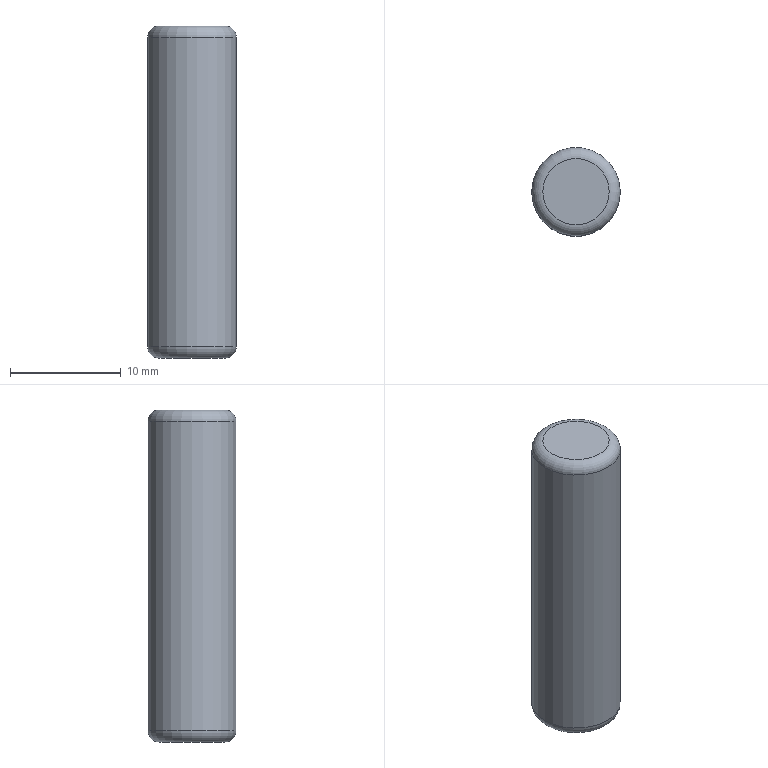Part | STEP file | 1 solid | 5 faces | box 8 x 8 x 30 mm | volume 1498 mm3 | plane 2 | torus 2 | cylinder 1 | commonest cylinder face diameters 8 x1
STEP:
#1=CARTESIAN_POINT('',(0.,0.,0.));
#2=DIRECTION('',(0.,0.,1.));
#3=DIRECTION('',(1.,0.,0.));
#4=AXIS2_PLACEMENT_3D('',#1,#2,#3);
#5=CARTESIAN_POINT('',(1623.549,352.48,33.619));
#6=VERTEX_POINT('',#5);
#7=CARTESIAN_POINT('',(1620.549,352.48,33.619));
#8=DIRECTION('',(0.,0.,-1.));
#9=DIRECTION('',(1.,0.,0.));
#10=AXIS2_PLACEMENT_3D('',#7,#8,#9);
#11=CIRCLE('',#10,3.);
#12=CARTESIAN_POINT('',(1620.549,352.48,33.619));
#13=DIRECTION('',(0.,0.,-1.));
#14=DIRECTION('',(-1.,0.,0.));
#15=AXIS2_PLACEMENT_3D('',#12,#13,#14);
#16=PLANE('',#15);
#17=CARTESIAN_POINT('',(0.,0.));
#18=DIRECTION('',(-1.,0.));
#19=AXIS2_PLACEMENT_2D('',#17,#18);
#20=CIRCLE('',#19,3.);
#21=(GEOMETRIC_REPRESENTATION_CONTEXT(2)PARAMETRIC_REPRESENTATION_CONTEXT()REPRESENTATION_CONTEXT('',''));
#22=DEFINITIONAL_REPRESENTATION('',(#20),#21);
#23=PCURVE('',#16,#22);
#24=CARTESIAN_POINT('',(1620.549,352.48,34.619));
#25=DIRECTION('',(0.,0.,-1.));
#26=DIRECTION('',(-1.,0.,0.));
#27=AXIS2_PLACEMENT_3D('',#24,#25,#26);
#28=TOROIDAL_SURFACE('',#27,3.,1.);
#29=CARTESIAN_POINT('',(3.142,7.854));
#30=DIRECTION('',(1.,0.));
#31=VECTOR('',#30,1.);
#32=LINE('',#29,#31);
#33=(GEOMETRIC_REPRESENTATION_CONTEXT(2)PARAMETRIC_REPRESENTATION_CONTEXT()REPRESENTATION_CONTEXT('',''));
#34=DEFINITIONAL_REPRESENTATION('',(#32),#33);
#35=PCURVE('',#28,#34);
#36=SURFACE_CURVE('',#11,(#23,#35),.PCURVE_S1.);
#37=EDGE_CURVE('',#6,#6,#36,.T.);
#38=ORIENTED_EDGE('',*,*,#37,.T.);
#39=EDGE_LOOP('',(#38));
#40=FACE_BOUND('',#39,.T.);
#41=ADVANCED_FACE('',(#40),#16,.T.);
#42=CARTESIAN_POINT('',(1617.549,352.48,63.619));
#43=VERTEX_POINT('',#42);
#44=CARTESIAN_POINT('',(1620.549,352.48,63.619));
#45=DIRECTION('',(0.,0.,1.));
#46=DIRECTION('',(-1.,0.,0.));
#47=AXIS2_PLACEMENT_3D('',#44,#45,#46);
#48=CIRCLE('',#47,3.);
#49=CARTESIAN_POINT('',(1620.549,352.48,63.619));
#50=DIRECTION('',(0.,0.,1.));
#51=DIRECTION('',(1.,0.,0.));
#52=AXIS2_PLACEMENT_3D('',#49,#50,#51);
#53=PLANE('',#52);
#54=CARTESIAN_POINT('',(0.,0.));
#55=DIRECTION('',(-1.,0.));
#56=AXIS2_PLACEMENT_2D('',#54,#55);
#57=CIRCLE('',#56,3.);
#58=(GEOMETRIC_REPRESENTATION_CONTEXT(2)PARAMETRIC_REPRESENTATION_CONTEXT()REPRESENTATION_CONTEXT('',''));
#59=DEFINITIONAL_REPRESENTATION('',(#57),#58);
#60=PCURVE('',#53,#59);
#61=CARTESIAN_POINT('',(1620.549,352.48,62.619));
#62=DIRECTION('',(0.,0.,1.));
#63=DIRECTION('',(1.,0.,0.));
#64=AXIS2_PLACEMENT_3D('',#61,#62,#63);
#65=TOROIDAL_SURFACE('',#64,3.,1.);
#66=CARTESIAN_POINT('',(3.142,7.854));
#67=DIRECTION('',(1.,0.));
#68=VECTOR('',#67,1.);
#69=LINE('',#66,#68);
#70=(GEOMETRIC_REPRESENTATION_CONTEXT(2)PARAMETRIC_REPRESENTATION_CONTEXT()REPRESENTATION_CONTEXT('',''));
#71=DEFINITIONAL_REPRESENTATION('',(#69),#70);
#72=PCURVE('',#65,#71);
#73=SURFACE_CURVE('',#48,(#60,#72),.PCURVE_S1.);
#74=EDGE_CURVE('',#43,#43,#73,.T.);
#75=ORIENTED_EDGE('',*,*,#74,.T.);
#76=EDGE_LOOP('',(#75));
#77=FACE_BOUND('',#76,.T.);
#78=ADVANCED_FACE('',(#77),#53,.T.);
#79=CARTESIAN_POINT('',(1616.549,352.48,62.619));
#80=VERTEX_POINT('',#79);
#81=CARTESIAN_POINT('',(1620.549,352.48,62.619));
#82=DIRECTION('',(0.,0.,-1.));
#83=DIRECTION('',(-1.,0.,0.));
#84=AXIS2_PLACEMENT_3D('',#81,#82,#83);
#85=CIRCLE('',#84,4.);
#86=CARTESIAN_POINT('',(1620.549,352.48,43.619));
#87=DIRECTION('',(0.,0.,-1.));
#88=DIRECTION('',(-1.,0.,0.));
#89=AXIS2_PLACEMENT_3D('',#86,#87,#88);
#90=CYLINDRICAL_SURFACE('',#89,4.);
#91=CARTESIAN_POINT('',(0.,-19.));
#92=DIRECTION('',(1.,0.));
#93=VECTOR('',#92,1.);
#94=LINE('',#91,#93);
#95=(GEOMETRIC_REPRESENTATION_CONTEXT(2)PARAMETRIC_REPRESENTATION_CONTEXT()REPRESENTATION_CONTEXT('',''));
#96=DEFINITIONAL_REPRESENTATION('',(#94),#95);
#97=PCURVE('',#90,#96);
#98=CARTESIAN_POINT('',(9.425,6.283));
#99=DIRECTION('',(-1.,0.));
#100=VECTOR('',#99,1.);
#101=LINE('',#98,#100);
#102=(GEOMETRIC_REPRESENTATION_CONTEXT(2)PARAMETRIC_REPRESENTATION_CONTEXT()REPRESENTATION_CONTEXT('',''));
#103=DEFINITIONAL_REPRESENTATION('',(#101),#102);
#104=PCURVE('',#65,#103);
#105=SURFACE_CURVE('',#85,(#97,#104),.PCURVE_S1.);
#106=EDGE_CURVE('',#80,#80,#105,.T.);
#107=ORIENTED_EDGE('',*,*,#106,.T.);
#108=CARTESIAN_POINT('',(1616.549,352.48,34.619));
#109=VERTEX_POINT('',#108);
#110=CARTESIAN_POINT('',(1616.549,352.48,62.619));
#111=CARTESIAN_POINT('',(1616.549,352.48,34.619));
#112=B_SPLINE_CURVE_WITH_KNOTS('',1,(#110,#111),.UNSPECIFIED.,.F.,.F.,(2,2),(-19.,9.),.PIECEWISE_BEZIER_KNOTS.);
#113=CARTESIAN_POINT('',(6.283,0.));
#114=DIRECTION('',(0.,1.));
#115=VECTOR('',#114,1.);
#116=LINE('',#113,#115);
#117=(GEOMETRIC_REPRESENTATION_CONTEXT(2)PARAMETRIC_REPRESENTATION_CONTEXT()REPRESENTATION_CONTEXT('',''));
#118=DEFINITIONAL_REPRESENTATION('',(#116),#117);
#119=PCURVE('',#90,#118);
#120=CARTESIAN_POINT('',(0.,0.));
#121=DIRECTION('',(0.,1.));
#122=VECTOR('',#121,1.);
#123=LINE('',#120,#122);
#124=(GEOMETRIC_REPRESENTATION_CONTEXT(2)PARAMETRIC_REPRESENTATION_CONTEXT()REPRESENTATION_CONTEXT('',''));
#125=DEFINITIONAL_REPRESENTATION('',(#123),#124);
#126=PCURVE('',#90,#125);
#127=SEAM_CURVE('',#112,(#119,#126),.PCURVE_S1.);
#128=EDGE_CURVE('',#80,#109,#127,.T.);
#129=ORIENTED_EDGE('',*,*,#128,.T.);
#130=CARTESIAN_POINT('',(1624.549,352.48,34.619));
#131=VERTEX_POINT('',#130);
#132=CARTESIAN_POINT('',(1620.549,352.48,34.619));
#133=DIRECTION('',(0.,0.,1.));
#134=DIRECTION('',(1.,0.,0.));
#135=AXIS2_PLACEMENT_3D('',#132,#133,#134);
#136=CIRCLE('',#135,4.);
#137=CARTESIAN_POINT('',(9.425,9.));
#138=DIRECTION('',(-1.,0.));
#139=VECTOR('',#138,1.);
#140=LINE('',#137,#139);
#141=(GEOMETRIC_REPRESENTATION_CONTEXT(2)PARAMETRIC_REPRESENTATION_CONTEXT()REPRESENTATION_CONTEXT('',''));
#142=DEFINITIONAL_REPRESENTATION('',(#140),#141);
#143=PCURVE('',#90,#142);
#144=CARTESIAN_POINT('',(9.425,6.283));
#145=DIRECTION('',(-1.,0.));
#146=VECTOR('',#145,1.);
#147=LINE('',#144,#146);
#148=(GEOMETRIC_REPRESENTATION_CONTEXT(2)PARAMETRIC_REPRESENTATION_CONTEXT()REPRESENTATION_CONTEXT('',''));
#149=DEFINITIONAL_REPRESENTATION('',(#147),#148);
#150=PCURVE('',#28,#149);
#151=SURFACE_CURVE('',#136,(#143,#150),.PCURVE_S1.);
#152=EDGE_CURVE('',#109,#131,#151,.T.);
#153=ORIENTED_EDGE('',*,*,#152,.T.);
#154=CARTESIAN_POINT('',(1620.549,352.48,34.619));
#155=DIRECTION('',(0.,0.,1.));
#156=DIRECTION('',(1.,0.,0.));
#157=AXIS2_PLACEMENT_3D('',#154,#155,#156);
#158=CIRCLE('',#157,4.);
#159=CARTESIAN_POINT('',(3.142,9.));
#160=DIRECTION('',(-1.,0.));
#161=VECTOR('',#160,1.);
#162=LINE('',#159,#161);
#163=(GEOMETRIC_REPRESENTATION_CONTEXT(2)PARAMETRIC_REPRESENTATION_CONTEXT()REPRESENTATION_CONTEXT('',''));
#164=DEFINITIONAL_REPRESENTATION('',(#162),#163);
#165=PCURVE('',#90,#164);
#166=CARTESIAN_POINT('',(9.425,6.283));
#167=DIRECTION('',(-1.,0.));
#168=VECTOR('',#167,1.);
#169=LINE('',#166,#168);
#170=(GEOMETRIC_REPRESENTATION_CONTEXT(2)PARAMETRIC_REPRESENTATION_CONTEXT()REPRESENTATION_CONTEXT('',''));
#171=DEFINITIONAL_REPRESENTATION('',(#169),#170);
#172=PCURVE('',#28,#171);
#173=SURFACE_CURVE('',#158,(#165,#172),.PCURVE_S1.);
#174=EDGE_CURVE('',#131,#109,#173,.T.);
#175=ORIENTED_EDGE('',*,*,#174,.T.);
#176=ORIENTED_EDGE('',*,*,#128,.F.);
#177=EDGE_LOOP('',(#107,#129,#153,#175,#176));
#178=FACE_BOUND('',#177,.T.);
#179=ADVANCED_FACE('',(#178),#90,.T.);
#180=ORIENTED_EDGE('',*,*,#74,.F.);
#181=CARTESIAN_POINT('',(1616.549,352.48,62.619));
#182=CARTESIAN_POINT('',(1616.549,352.48,62.886));
#183=CARTESIAN_POINT('',(1616.634,352.48,63.147));
#184=CARTESIAN_POINT('',(1616.797,352.48,63.371));
#185=CARTESIAN_POINT('',(1617.021,352.48,63.534));
#186=CARTESIAN_POINT('',(1617.282,352.48,63.619));
#187=CARTESIAN_POINT('',(1617.549,352.48,63.619));
#188=(BOUNDED_CURVE()B_SPLINE_CURVE(6,(#181,#182,#183,#184,#185,#186,#187),.UNSPECIFIED.,.F.,.F.)B_SPLINE_CURVE_WITH_KNOTS((7,7),(0.,1.571),.PIECEWISE_BEZIER_KNOTS.)CURVE()GEOMETRIC_REPRESENTATION_ITEM()RATIONAL_B_SPLINE_CURVE((1.031,1.01,0.9979,0.994,0.9979,1.01,1.031))REPRESENTATION_ITEM(''));
#189=CARTESIAN_POINT('',(3.142,6.283));
#190=DIRECTION('',(0.,1.));
#191=VECTOR('',#190,1.);
#192=LINE('',#189,#191);
#193=(GEOMETRIC_REPRESENTATION_CONTEXT(2)PARAMETRIC_REPRESENTATION_CONTEXT()REPRESENTATION_CONTEXT('',''));
#194=DEFINITIONAL_REPRESENTATION('',(#192),#193);
#195=PCURVE('',#65,#194);
#196=CARTESIAN_POINT('',(9.425,6.283));
#197=DIRECTION('',(0.,1.));
#198=VECTOR('',#197,1.);
#199=LINE('',#196,#198);
#200=(GEOMETRIC_REPRESENTATION_CONTEXT(2)PARAMETRIC_REPRESENTATION_CONTEXT()REPRESENTATION_CONTEXT('',''));
#201=DEFINITIONAL_REPRESENTATION('',(#199),#200);
#202=PCURVE('',#65,#201);
#203=SEAM_CURVE('',#188,(#195,#202),.PCURVE_S1.);
#204=EDGE_CURVE('',#80,#43,#203,.T.);
#205=ORIENTED_EDGE('',*,*,#204,.F.);
#206=ORIENTED_EDGE('',*,*,#106,.F.);
#207=ORIENTED_EDGE('',*,*,#204,.T.);
#208=EDGE_LOOP('',(#180,#205,#206,#207));
#209=FACE_BOUND('',#208,.T.);
#210=ADVANCED_FACE('',(#209),#65,.T.);
#211=ORIENTED_EDGE('',*,*,#37,.F.);
#212=CARTESIAN_POINT('',(1624.549,352.48,34.619));
#213=CARTESIAN_POINT('',(1624.549,352.48,34.352));
#214=CARTESIAN_POINT('',(1624.464,352.48,34.091));
#215=CARTESIAN_POINT('',(1624.301,352.48,33.867));
#216=CARTESIAN_POINT('',(1624.077,352.48,33.704));
#217=CARTESIAN_POINT('',(1623.817,352.48,33.619));
#218=CARTESIAN_POINT('',(1623.549,352.48,33.619));
#219=(BOUNDED_CURVE()B_SPLINE_CURVE(6,(#212,#213,#214,#215,#216,#217,#218),.UNSPECIFIED.,.F.,.F.)B_SPLINE_CURVE_WITH_KNOTS((7,7),(0.,1.571),.PIECEWISE_BEZIER_KNOTS.)CURVE()GEOMETRIC_REPRESENTATION_ITEM()RATIONAL_B_SPLINE_CURVE((1.031,1.01,0.9979,0.994,0.9979,1.01,1.031))REPRESENTATION_ITEM(''));
#220=CARTESIAN_POINT('',(3.142,6.283));
#221=DIRECTION('',(0.,1.));
#222=VECTOR('',#221,1.);
#223=LINE('',#220,#222);
#224=(GEOMETRIC_REPRESENTATION_CONTEXT(2)PARAMETRIC_REPRESENTATION_CONTEXT()REPRESENTATION_CONTEXT('',''));
#225=DEFINITIONAL_REPRESENTATION('',(#223),#224);
#226=PCURVE('',#28,#225);
#227=CARTESIAN_POINT('',(9.425,6.283));
#228=DIRECTION('',(0.,1.));
#229=VECTOR('',#228,1.);
#230=LINE('',#227,#229);
#231=(GEOMETRIC_REPRESENTATION_CONTEXT(2)PARAMETRIC_REPRESENTATION_CONTEXT()REPRESENTATION_CONTEXT('',''));
#232=DEFINITIONAL_REPRESENTATION('',(#230),#231);
#233=PCURVE('',#28,#232);
#234=SEAM_CURVE('',#219,(#226,#233),.PCURVE_S1.);
#235=EDGE_CURVE('',#131,#6,#234,.T.);
#236=ORIENTED_EDGE('',*,*,#235,.F.);
#237=ORIENTED_EDGE('',*,*,#152,.F.);
#238=ORIENTED_EDGE('',*,*,#174,.F.);
#239=ORIENTED_EDGE('',*,*,#235,.T.);
#240=EDGE_LOOP('',(#211,#236,#237,#238,#239));
#241=FACE_BOUND('',#240,.T.);
#242=ADVANCED_FACE('',(#241),#28,.T.);
#243=CLOSED_SHELL('',(#41,#78,#179,#210,#242));
#244=MANIFOLD_SOLID_BREP('',#243);
#245=(LENGTH_UNIT()NAMED_UNIT(*)SI_UNIT(.MILLI.,.METRE.));
#246=UNCERTAINTY_MEASURE_WITH_UNIT(LENGTH_MEASURE(0.00001),#245,'','');
#247=(NAMED_UNIT(*)PLANE_ANGLE_UNIT()SI_UNIT($,.RADIAN.));
#248=(NAMED_UNIT(*)SI_UNIT($,.STERADIAN.)SOLID_ANGLE_UNIT());
#249=(GEOMETRIC_REPRESENTATION_CONTEXT(3)GLOBAL_UNCERTAINTY_ASSIGNED_CONTEXT((#246))GLOBAL_UNIT_ASSIGNED_CONTEXT((#245,#247,#248))REPRESENTATION_CONTEXT('',''));
#250=ADVANCED_BREP_SHAPE_REPRESENTATION('',(#4,#244),#249);